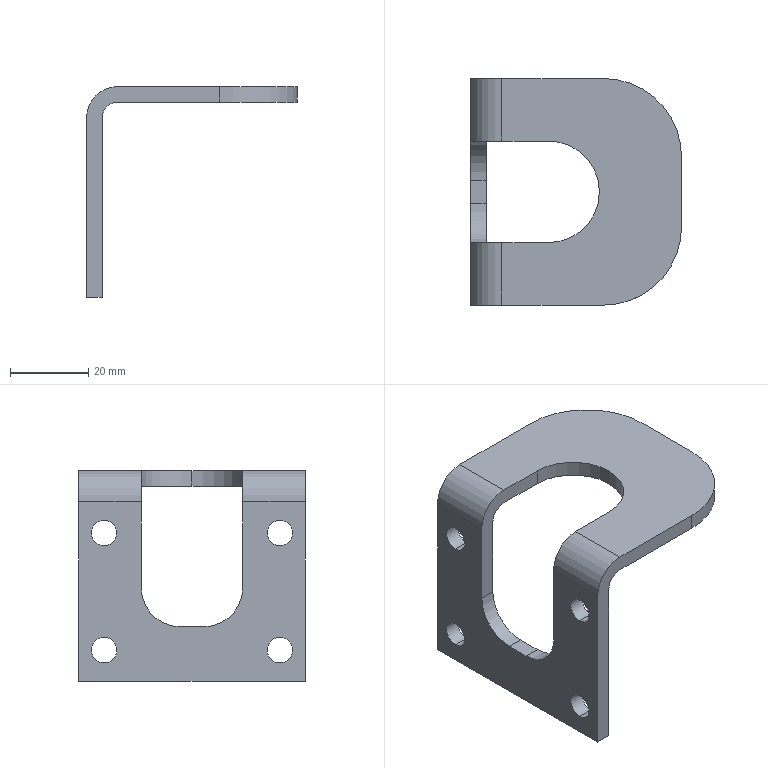Part | STEP file | X77-02002 | 1 solid | 29 faces | box 54 x 58 x 54 mm | volume 15867 mm3 | cylinder 18 | plane 11 | commonest cylinder face diameters 6.5 x8 8 x2 16 x2 20 x2 26 x2 40 x2
STEP:
#1=CARTESIAN_POINT('',(-63.245,51.5,31.345));
#2=VERTEX_POINT('',#1);
#3=CARTESIAN_POINT('',(-63.245,51.5,24.845));
#4=VERTEX_POINT('',#3);
#5=CARTESIAN_POINT('',(-63.245,51.5,28.095));
#6=DIRECTION('',(1.,0.,0.));
#7=DIRECTION('',(0.,0.,-1.));
#8=AXIS2_PLACEMENT_3D('',#5,#6,#7);
#9=CIRCLE('',#8,3.25);
#10=EDGE_CURVE('',#2,#4,#9,.T.);
#11=ORIENTED_EDGE('',*,*,#10,.F.);
#12=CARTESIAN_POINT('',(-59.245,51.5,31.345));
#13=VERTEX_POINT('',#12);
#14=CARTESIAN_POINT('',(-69.245,51.5,31.345));
#15=DIRECTION('',(1.,0.,0.));
#16=VECTOR('',#15,1000.);
#17=LINE('',#14,#16);
#18=EDGE_CURVE('',#2,#13,#17,.T.);
#19=ORIENTED_EDGE('',*,*,#18,.T.);
#20=CARTESIAN_POINT('',(-59.245,51.5,24.845));
#21=VERTEX_POINT('',#20);
#22=CARTESIAN_POINT('',(-59.245,51.5,28.095));
#23=DIRECTION('',(1.,0.,0.));
#24=DIRECTION('',(0.,0.,-1.));
#25=AXIS2_PLACEMENT_3D('',#22,#23,#24);
#26=CIRCLE('',#25,3.25);
#27=EDGE_CURVE('',#13,#21,#26,.T.);
#28=ORIENTED_EDGE('',*,*,#27,.T.);
#29=CARTESIAN_POINT('',(-69.245,51.5,24.845));
#30=DIRECTION('',(1.,0.,0.));
#31=VECTOR('',#30,1000.);
#32=LINE('',#29,#31);
#33=EDGE_CURVE('',#4,#21,#32,.T.);
#34=ORIENTED_EDGE('',*,*,#33,.F.);
#35=EDGE_LOOP('',(#11,#19,#28,#34));
#36=FACE_OUTER_BOUND('',#35,.T.);
#37=CARTESIAN_POINT('',(-69.245,51.5,28.095));
#38=DIRECTION('',(1.,0.,0.));
#39=DIRECTION('',(0.,0.,-1.));
#40=AXIS2_PLACEMENT_3D('',#37,#38,#39);
#41=CYLINDRICAL_SURFACE('',#40,3.25);
#42=ADVANCED_FACE('',(#36),#41,.F.);
#43=CARTESIAN_POINT('',(-63.245,6.5,31.345));
#44=VERTEX_POINT('',#43);
#45=CARTESIAN_POINT('',(-63.245,6.5,24.845));
#46=VERTEX_POINT('',#45);
#47=CARTESIAN_POINT('',(-63.245,6.5,28.095));
#48=DIRECTION('',(1.,0.,0.));
#49=DIRECTION('',(0.,0.,-1.));
#50=AXIS2_PLACEMENT_3D('',#47,#48,#49);
#51=CIRCLE('',#50,3.25);
#52=EDGE_CURVE('',#44,#46,#51,.T.);
#53=ORIENTED_EDGE('',*,*,#52,.F.);
#54=CARTESIAN_POINT('',(-59.245,6.5,31.345));
#55=VERTEX_POINT('',#54);
#56=CARTESIAN_POINT('',(-69.245,6.5,31.345));
#57=DIRECTION('',(1.,0.,0.));
#58=VECTOR('',#57,1000.);
#59=LINE('',#56,#58);
#60=EDGE_CURVE('',#44,#55,#59,.T.);
#61=ORIENTED_EDGE('',*,*,#60,.T.);
#62=CARTESIAN_POINT('',(-59.245,6.5,24.845));
#63=VERTEX_POINT('',#62);
#64=CARTESIAN_POINT('',(-59.245,6.5,28.095));
#65=DIRECTION('',(1.,0.,0.));
#66=DIRECTION('',(0.,0.,-1.));
#67=AXIS2_PLACEMENT_3D('',#64,#65,#66);
#68=CIRCLE('',#67,3.25);
#69=EDGE_CURVE('',#55,#63,#68,.T.);
#70=ORIENTED_EDGE('',*,*,#69,.T.);
#71=CARTESIAN_POINT('',(-69.245,6.5,24.845));
#72=DIRECTION('',(1.,0.,0.));
#73=VECTOR('',#72,1000.);
#74=LINE('',#71,#73);
#75=EDGE_CURVE('',#46,#63,#74,.T.);
#76=ORIENTED_EDGE('',*,*,#75,.F.);
#77=EDGE_LOOP('',(#53,#61,#70,#76));
#78=FACE_OUTER_BOUND('',#77,.T.);
#79=CARTESIAN_POINT('',(-69.245,6.5,28.095));
#80=DIRECTION('',(1.,0.,0.));
#81=DIRECTION('',(0.,0.,-1.));
#82=AXIS2_PLACEMENT_3D('',#79,#80,#81);
#83=CYLINDRICAL_SURFACE('',#82,3.25);
#84=ADVANCED_FACE('',(#78),#83,.F.);
#85=CARTESIAN_POINT('',(-63.245,6.5,1.345));
#86=VERTEX_POINT('',#85);
#87=CARTESIAN_POINT('',(-63.245,6.5,-5.155));
#88=VERTEX_POINT('',#87);
#89=CARTESIAN_POINT('',(-63.245,6.5,-1.905));
#90=DIRECTION('',(1.,0.,0.));
#91=DIRECTION('',(0.,0.,-1.));
#92=AXIS2_PLACEMENT_3D('',#89,#90,#91);
#93=CIRCLE('',#92,3.25);
#94=EDGE_CURVE('',#86,#88,#93,.T.);
#95=ORIENTED_EDGE('',*,*,#94,.F.);
#96=CARTESIAN_POINT('',(-59.245,6.5,1.345));
#97=VERTEX_POINT('',#96);
#98=CARTESIAN_POINT('',(-69.245,6.5,1.345));
#99=DIRECTION('',(1.,0.,0.));
#100=VECTOR('',#99,1000.);
#101=LINE('',#98,#100);
#102=EDGE_CURVE('',#86,#97,#101,.T.);
#103=ORIENTED_EDGE('',*,*,#102,.T.);
#104=CARTESIAN_POINT('',(-59.245,6.5,-5.155));
#105=VERTEX_POINT('',#104);
#106=CARTESIAN_POINT('',(-59.245,6.5,-1.905));
#107=DIRECTION('',(1.,0.,0.));
#108=DIRECTION('',(0.,0.,-1.));
#109=AXIS2_PLACEMENT_3D('',#106,#107,#108);
#110=CIRCLE('',#109,3.25);
#111=EDGE_CURVE('',#97,#105,#110,.T.);
#112=ORIENTED_EDGE('',*,*,#111,.T.);
#113=CARTESIAN_POINT('',(-69.245,6.5,-5.155));
#114=DIRECTION('',(1.,0.,0.));
#115=VECTOR('',#114,1000.);
#116=LINE('',#113,#115);
#117=EDGE_CURVE('',#88,#105,#116,.T.);
#118=ORIENTED_EDGE('',*,*,#117,.F.);
#119=EDGE_LOOP('',(#95,#103,#112,#118));
#120=FACE_OUTER_BOUND('',#119,.T.);
#121=CARTESIAN_POINT('',(-69.245,6.5,-1.905));
#122=DIRECTION('',(1.,0.,0.));
#123=DIRECTION('',(0.,0.,-1.));
#124=AXIS2_PLACEMENT_3D('',#121,#122,#123);
#125=CYLINDRICAL_SURFACE('',#124,3.25);
#126=ADVANCED_FACE('',(#120),#125,.F.);
#127=CARTESIAN_POINT('',(-63.245,51.5,1.345));
#128=VERTEX_POINT('',#127);
#129=CARTESIAN_POINT('',(-63.245,51.5,-5.155));
#130=VERTEX_POINT('',#129);
#131=CARTESIAN_POINT('',(-63.245,51.5,-1.905));
#132=DIRECTION('',(1.,0.,0.));
#133=DIRECTION('',(0.,0.,-1.));
#134=AXIS2_PLACEMENT_3D('',#131,#132,#133);
#135=CIRCLE('',#134,3.25);
#136=EDGE_CURVE('',#128,#130,#135,.T.);
#137=ORIENTED_EDGE('',*,*,#136,.F.);
#138=CARTESIAN_POINT('',(-59.245,51.5,1.345));
#139=VERTEX_POINT('',#138);
#140=CARTESIAN_POINT('',(-69.245,51.5,1.345));
#141=DIRECTION('',(1.,0.,0.));
#142=VECTOR('',#141,1000.);
#143=LINE('',#140,#142);
#144=EDGE_CURVE('',#128,#139,#143,.T.);
#145=ORIENTED_EDGE('',*,*,#144,.T.);
#146=CARTESIAN_POINT('',(-59.245,51.5,-5.155));
#147=VERTEX_POINT('',#146);
#148=CARTESIAN_POINT('',(-59.245,51.5,-1.905));
#149=DIRECTION('',(1.,0.,0.));
#150=DIRECTION('',(0.,0.,-1.));
#151=AXIS2_PLACEMENT_3D('',#148,#149,#150);
#152=CIRCLE('',#151,3.25);
#153=EDGE_CURVE('',#139,#147,#152,.T.);
#154=ORIENTED_EDGE('',*,*,#153,.T.);
#155=CARTESIAN_POINT('',(-69.245,51.5,-5.155));
#156=DIRECTION('',(1.,0.,0.));
#157=VECTOR('',#156,1000.);
#158=LINE('',#155,#157);
#159=EDGE_CURVE('',#130,#147,#158,.T.);
#160=ORIENTED_EDGE('',*,*,#159,.F.);
#161=EDGE_LOOP('',(#137,#145,#154,#160));
#162=FACE_OUTER_BOUND('',#161,.T.);
#163=CARTESIAN_POINT('',(-69.245,51.5,-1.905));
#164=DIRECTION('',(1.,0.,0.));
#165=DIRECTION('',(0.,0.,-1.));
#166=AXIS2_PLACEMENT_3D('',#163,#164,#165);
#167=CYLINDRICAL_SURFACE('',#166,3.25);
#168=ADVANCED_FACE('',(#162),#167,.F.);
#169=CARTESIAN_POINT('',(-30.245,29.,40.095));
#170=VERTEX_POINT('',#169);
#171=CARTESIAN_POINT('',(-43.245,42.,40.095));
#172=VERTEX_POINT('',#171);
#173=CARTESIAN_POINT('',(-43.245,29.,40.095));
#174=DIRECTION('',(0.,0.,1.));
#175=DIRECTION('',(1.,0.,0.));
#176=AXIS2_PLACEMENT_3D('',#173,#174,#175);
#177=CIRCLE('',#176,13.);
#178=EDGE_CURVE('',#170,#172,#177,.T.);
#179=ORIENTED_EDGE('',*,*,#178,.F.);
#180=CARTESIAN_POINT('',(-30.245,29.,44.095));
#181=VERTEX_POINT('',#180);
#182=CARTESIAN_POINT('',(-30.245,29.,4.095));
#183=DIRECTION('',(0.,0.,1.));
#184=VECTOR('',#183,1000.);
#185=LINE('',#182,#184);
#186=EDGE_CURVE('',#170,#181,#185,.T.);
#187=ORIENTED_EDGE('',*,*,#186,.T.);
#188=CARTESIAN_POINT('',(-43.245,42.,44.095));
#189=VERTEX_POINT('',#188);
#190=CARTESIAN_POINT('',(-43.245,29.,44.095));
#191=DIRECTION('',(0.,0.,1.));
#192=DIRECTION('',(1.,0.,0.));
#193=AXIS2_PLACEMENT_3D('',#190,#191,#192);
#194=CIRCLE('',#193,13.);
#195=EDGE_CURVE('',#181,#189,#194,.T.);
#196=ORIENTED_EDGE('',*,*,#195,.T.);
#197=CARTESIAN_POINT('',(-43.245,42.,4.095));
#198=DIRECTION('',(0.,0.,1.));
#199=VECTOR('',#198,1000.);
#200=LINE('',#197,#199);
#201=EDGE_CURVE('',#172,#189,#200,.T.);
#202=ORIENTED_EDGE('',*,*,#201,.F.);
#203=EDGE_LOOP('',(#179,#187,#196,#202));
#204=FACE_OUTER_BOUND('',#203,.T.);
#205=CARTESIAN_POINT('',(-43.245,29.,4.095));
#206=DIRECTION('',(0.,0.,1.));
#207=DIRECTION('',(1.,0.,0.));
#208=AXIS2_PLACEMENT_3D('',#205,#206,#207);
#209=CYLINDRICAL_SURFACE('',#208,13.);
#210=ADVANCED_FACE('',(#204),#209,.F.);
#211=CARTESIAN_POINT('',(-63.245,58.,36.095));
#212=VERTEX_POINT('',#211);
#213=CARTESIAN_POINT('',(-63.245,42.,36.095));
#214=VERTEX_POINT('',#213);
#215=CARTESIAN_POINT('',(-63.245,58.,36.095));
#216=DIRECTION('',(0.,-1.,0.));
#217=VECTOR('',#216,1000.);
#218=LINE('',#215,#217);
#219=EDGE_CURVE('',#212,#214,#218,.T.);
#220=ORIENTED_EDGE('',*,*,#219,.T.);
#221=CARTESIAN_POINT('',(-55.245,42.,44.095));
#222=VERTEX_POINT('',#221);
#223=CARTESIAN_POINT('',(-55.245,42.,36.095));
#224=DIRECTION('',(0.,1.,0.));
#225=DIRECTION('',(0.,0.,1.));
#226=AXIS2_PLACEMENT_3D('',#223,#224,#225);
#227=CIRCLE('',#226,8.);
#228=EDGE_CURVE('',#214,#222,#227,.T.);
#229=ORIENTED_EDGE('',*,*,#228,.T.);
#230=CARTESIAN_POINT('',(-55.245,58.,44.095));
#231=VERTEX_POINT('',#230);
#232=CARTESIAN_POINT('',(-55.245,58.,44.095));
#233=DIRECTION('',(0.,-1.,0.));
#234=VECTOR('',#233,1000.);
#235=LINE('',#232,#234);
#236=EDGE_CURVE('',#231,#222,#235,.T.);
#237=ORIENTED_EDGE('',*,*,#236,.F.);
#238=CARTESIAN_POINT('',(-55.245,58.,36.095));
#239=DIRECTION('',(0.,1.,0.));
#240=DIRECTION('',(0.,0.,-1.));
#241=AXIS2_PLACEMENT_3D('',#238,#239,#240);
#242=CIRCLE('',#241,8.);
#243=EDGE_CURVE('',#212,#231,#242,.T.);
#244=ORIENTED_EDGE('',*,*,#243,.F.);
#245=EDGE_LOOP('',(#220,#229,#237,#244));
#246=FACE_OUTER_BOUND('',#245,.T.);
#247=CARTESIAN_POINT('',(-55.245,58.,36.095));
#248=DIRECTION('',(0.,-1.,0.));
#249=DIRECTION('',(0.,0.,-1.));
#250=AXIS2_PLACEMENT_3D('',#247,#248,#249);
#251=CYLINDRICAL_SURFACE('',#250,8.);
#252=ADVANCED_FACE('',(#246),#251,.T.);
#253=CARTESIAN_POINT('',(-55.245,58.,40.095));
#254=VERTEX_POINT('',#253);
#255=CARTESIAN_POINT('',(-55.245,42.,40.095));
#256=VERTEX_POINT('',#255);
#257=CARTESIAN_POINT('',(-55.245,58.,40.095));
#258=DIRECTION('',(0.,-1.,0.));
#259=VECTOR('',#258,1000.);
#260=LINE('',#257,#259);
#261=EDGE_CURVE('',#254,#256,#260,.T.);
#262=ORIENTED_EDGE('',*,*,#261,.T.);
#263=CARTESIAN_POINT('',(-59.245,42.,36.095));
#264=VERTEX_POINT('',#263);
#265=CARTESIAN_POINT('',(-55.245,42.,36.095));
#266=DIRECTION('',(0.,-1.,0.));
#267=DIRECTION('',(0.,0.,1.));
#268=AXIS2_PLACEMENT_3D('',#265,#266,#267);
#269=CIRCLE('',#268,4.);
#270=EDGE_CURVE('',#256,#264,#269,.T.);
#271=ORIENTED_EDGE('',*,*,#270,.T.);
#272=CARTESIAN_POINT('',(-59.245,58.,36.095));
#273=VERTEX_POINT('',#272);
#274=CARTESIAN_POINT('',(-59.245,58.,36.095));
#275=DIRECTION('',(0.,-1.,0.));
#276=VECTOR('',#275,1000.);
#277=LINE('',#274,#276);
#278=EDGE_CURVE('',#273,#264,#277,.T.);
#279=ORIENTED_EDGE('',*,*,#278,.F.);
#280=CARTESIAN_POINT('',(-55.245,58.,36.095));
#281=DIRECTION('',(0.,-1.,0.));
#282=DIRECTION('',(0.,0.,-1.));
#283=AXIS2_PLACEMENT_3D('',#280,#281,#282);
#284=CIRCLE('',#283,4.);
#285=EDGE_CURVE('',#254,#273,#284,.T.);
#286=ORIENTED_EDGE('',*,*,#285,.F.);
#287=EDGE_LOOP('',(#262,#271,#279,#286));
#288=FACE_OUTER_BOUND('',#287,.T.);
#289=CARTESIAN_POINT('',(-55.245,58.,36.095));
#290=DIRECTION('',(0.,-1.,0.));
#291=DIRECTION('',(0.,0.,-1.));
#292=AXIS2_PLACEMENT_3D('',#289,#290,#291);
#293=CYLINDRICAL_SURFACE('',#292,4.);
#294=ADVANCED_FACE('',(#288),#293,.F.);
#295=CARTESIAN_POINT('',(-59.245,0.,-9.905));
#296=VERTEX_POINT('',#295);
#297=CARTESIAN_POINT('',(-63.245,0.,-9.905));
#298=VERTEX_POINT('',#297);
#299=CARTESIAN_POINT('',(-59.245,0.,-9.905));
#300=DIRECTION('',(-1.,0.,0.));
#301=VECTOR('',#300,1000.);
#302=LINE('',#299,#301);
#303=EDGE_CURVE('',#296,#298,#302,.T.);
#304=ORIENTED_EDGE('',*,*,#303,.T.);
#305=CARTESIAN_POINT('',(-63.245,58.,-9.905));
#306=VERTEX_POINT('',#305);
#307=CARTESIAN_POINT('',(-63.245,58.,-9.905));
#308=DIRECTION('',(0.,-1.,0.));
#309=VECTOR('',#308,1000.);
#310=LINE('',#307,#309);
#311=EDGE_CURVE('',#306,#298,#310,.T.);
#312=ORIENTED_EDGE('',*,*,#311,.F.);
#313=CARTESIAN_POINT('',(-59.245,58.,-9.905));
#314=VERTEX_POINT('',#313);
#315=CARTESIAN_POINT('',(-59.245,58.,-9.905));
#316=DIRECTION('',(-1.,0.,0.));
#317=VECTOR('',#316,1000.);
#318=LINE('',#315,#317);
#319=EDGE_CURVE('',#314,#306,#318,.T.);
#320=ORIENTED_EDGE('',*,*,#319,.F.);
#321=CARTESIAN_POINT('',(-59.245,58.,-9.905));
#322=DIRECTION('',(0.,-1.,0.));
#323=VECTOR('',#322,1000.);
#324=LINE('',#321,#323);
#325=EDGE_CURVE('',#314,#296,#324,.T.);
#326=ORIENTED_EDGE('',*,*,#325,.T.);
#327=EDGE_LOOP('',(#304,#312,#320,#326));
#328=FACE_OUTER_BOUND('',#327,.T.);
#329=CARTESIAN_POINT('',(-59.245,58.,-9.905));
#330=DIRECTION('',(0.,0.,1.));
#331=DIRECTION('',(1.,0.,0.));
#332=AXIS2_PLACEMENT_3D('',#329,#330,#331);
#333=PLANE('',#332);
#334=ADVANCED_FACE('',(#328),#333,.F.);
#335=CARTESIAN_POINT('',(-63.245,51.5,28.095));
#336=DIRECTION('',(1.,0.,0.));
#337=DIRECTION('',(0.,0.,-1.));
#338=AXIS2_PLACEMENT_3D('',#335,#336,#337);
#339=CIRCLE('',#338,3.25);
#340=EDGE_CURVE('',#4,#2,#339,.T.);
#341=ORIENTED_EDGE('',*,*,#340,.T.);
#342=ORIENTED_EDGE('',*,*,#10,.T.);
#343=EDGE_LOOP('',(#341,#342));
#344=FACE_BOUND('',#343,.T.);
#345=CARTESIAN_POINT('',(-63.245,6.5,28.095));
#346=DIRECTION('',(1.,0.,0.));
#347=DIRECTION('',(0.,0.,-1.));
#348=AXIS2_PLACEMENT_3D('',#345,#346,#347);
#349=CIRCLE('',#348,3.25);
#350=EDGE_CURVE('',#46,#44,#349,.T.);
#351=ORIENTED_EDGE('',*,*,#350,.T.);
#352=ORIENTED_EDGE('',*,*,#52,.T.);
#353=EDGE_LOOP('',(#351,#352));
#354=FACE_BOUND('',#353,.T.);
#355=CARTESIAN_POINT('',(-63.245,6.5,-1.905));
#356=DIRECTION('',(1.,0.,0.));
#357=DIRECTION('',(0.,0.,-1.));
#358=AXIS2_PLACEMENT_3D('',#355,#356,#357);
#359=CIRCLE('',#358,3.25);
#360=EDGE_CURVE('',#88,#86,#359,.T.);
#361=ORIENTED_EDGE('',*,*,#360,.T.);
#362=ORIENTED_EDGE('',*,*,#94,.T.);
#363=EDGE_LOOP('',(#361,#362));
#364=FACE_BOUND('',#363,.T.);
#365=CARTESIAN_POINT('',(-63.245,51.5,-1.905));
#366=DIRECTION('',(1.,0.,0.));
#367=DIRECTION('',(0.,0.,-1.));
#368=AXIS2_PLACEMENT_3D('',#365,#366,#367);
#369=CIRCLE('',#368,3.25);
#370=EDGE_CURVE('',#130,#128,#369,.T.);
#371=ORIENTED_EDGE('',*,*,#370,.T.);
#372=ORIENTED_EDGE('',*,*,#136,.T.);
#373=EDGE_LOOP('',(#371,#372));
#374=FACE_BOUND('',#373,.T.);
#375=CARTESIAN_POINT('',(-63.245,32.,4.095));
#376=VERTEX_POINT('',#375);
#377=CARTESIAN_POINT('',(-63.245,26.,4.095));
#378=VERTEX_POINT('',#377);
#379=CARTESIAN_POINT('',(-63.245,58.,4.095));
#380=DIRECTION('',(0.,-1.,0.));
#381=VECTOR('',#380,1000.);
#382=LINE('',#379,#381);
#383=EDGE_CURVE('',#376,#378,#382,.T.);
#384=ORIENTED_EDGE('',*,*,#383,.F.);
#385=CARTESIAN_POINT('',(-63.245,42.,14.095));
#386=VERTEX_POINT('',#385);
#387=CARTESIAN_POINT('',(-63.245,32.,14.095));
#388=DIRECTION('',(1.,0.,0.));
#389=DIRECTION('',(0.,0.,-1.));
#390=AXIS2_PLACEMENT_3D('',#387,#388,#389);
#391=CIRCLE('',#390,10.);
#392=EDGE_CURVE('',#376,#386,#391,.T.);
#393=ORIENTED_EDGE('',*,*,#392,.T.);
#394=CARTESIAN_POINT('',(-63.245,42.,4.095));
#395=DIRECTION('',(0.,0.,1.));
#396=VECTOR('',#395,1000.);
#397=LINE('',#394,#396);
#398=EDGE_CURVE('',#386,#214,#397,.T.);
#399=ORIENTED_EDGE('',*,*,#398,.T.);
#400=ORIENTED_EDGE('',*,*,#219,.F.);
#401=CARTESIAN_POINT('',(-63.245,58.,-9.905));
#402=DIRECTION('',(0.,0.,1.));
#403=VECTOR('',#402,1000.);
#404=LINE('',#401,#403);
#405=EDGE_CURVE('',#306,#212,#404,.T.);
#406=ORIENTED_EDGE('',*,*,#405,.F.);
#407=ORIENTED_EDGE('',*,*,#311,.T.);
#408=CARTESIAN_POINT('',(-63.245,0.,36.095));
#409=VERTEX_POINT('',#408);
#410=CARTESIAN_POINT('',(-63.245,0.,-9.905));
#411=DIRECTION('',(0.,0.,1.));
#412=VECTOR('',#411,1000.);
#413=LINE('',#410,#412);
#414=EDGE_CURVE('',#298,#409,#413,.T.);
#415=ORIENTED_EDGE('',*,*,#414,.T.);
#416=CARTESIAN_POINT('',(-63.245,16.,36.095));
#417=VERTEX_POINT('',#416);
#418=CARTESIAN_POINT('',(-63.245,58.,36.095));
#419=DIRECTION('',(0.,-1.,0.));
#420=VECTOR('',#419,1000.);
#421=LINE('',#418,#420);
#422=EDGE_CURVE('',#417,#409,#421,.T.);
#423=ORIENTED_EDGE('',*,*,#422,.F.);
#424=CARTESIAN_POINT('',(-63.245,16.,14.095));
#425=VERTEX_POINT('',#424);
#426=CARTESIAN_POINT('',(-63.245,16.,4.095));
#427=DIRECTION('',(0.,0.,1.));
#428=VECTOR('',#427,1000.);
#429=LINE('',#426,#428);
#430=EDGE_CURVE('',#425,#417,#429,.T.);
#431=ORIENTED_EDGE('',*,*,#430,.F.);
#432=CARTESIAN_POINT('',(-63.245,26.,14.095));
#433=DIRECTION('',(1.,0.,0.));
#434=DIRECTION('',(0.,0.,-1.));
#435=AXIS2_PLACEMENT_3D('',#432,#433,#434);
#436=CIRCLE('',#435,10.);
#437=EDGE_CURVE('',#425,#378,#436,.T.);
#438=ORIENTED_EDGE('',*,*,#437,.T.);
#439=EDGE_LOOP('',(#384,#393,#399,#400,#406,#407,#415,#423,#431,#438));
#440=FACE_OUTER_BOUND('',#439,.T.);
#441=CARTESIAN_POINT('',(-63.245,58.,-9.905));
#442=DIRECTION('',(1.,0.,0.));
#443=DIRECTION('',(0.,0.,-1.));
#444=AXIS2_PLACEMENT_3D('',#441,#442,#443);
#445=PLANE('',#444);
#446=ADVANCED_FACE('',(#344,#354,#364,#374,#440),#445,.F.);
#447=CARTESIAN_POINT('',(-55.245,16.,44.095));
#448=VERTEX_POINT('',#447);
#449=CARTESIAN_POINT('',(-55.245,0.,44.095));
#450=VERTEX_POINT('',#449);
#451=CARTESIAN_POINT('',(-55.245,58.,44.095));
#452=DIRECTION('',(0.,-1.,0.));
#453=VECTOR('',#452,1000.);
#454=LINE('',#451,#453);
#455=EDGE_CURVE('',#448,#450,#454,.T.);
#456=ORIENTED_EDGE('',*,*,#455,.F.);
#457=CARTESIAN_POINT('',(-55.245,16.,36.095));
#458=DIRECTION('',(0.,-1.,0.));
#459=DIRECTION('',(0.,0.,-1.));
#460=AXIS2_PLACEMENT_3D('',#457,#458,#459);
#461=CIRCLE('',#460,8.);
#462=EDGE_CURVE('',#448,#417,#461,.T.);
#463=ORIENTED_EDGE('',*,*,#462,.T.);
#464=ORIENTED_EDGE('',*,*,#422,.T.);
#465=CARTESIAN_POINT('',(-55.245,0.,36.095));
#466=DIRECTION('',(0.,1.,0.));
#467=DIRECTION('',(0.,0.,-1.));
#468=AXIS2_PLACEMENT_3D('',#465,#466,#467);
#469=CIRCLE('',#468,8.);
#470=EDGE_CURVE('',#409,#450,#469,.T.);
#471=ORIENTED_EDGE('',*,*,#470,.T.);
#472=EDGE_LOOP('',(#456,#463,#464,#471));
#473=FACE_OUTER_BOUND('',#472,.T.);
#474=CARTESIAN_POINT('',(-55.245,58.,36.095));
#475=DIRECTION('',(0.,-1.,0.));
#476=DIRECTION('',(0.,0.,-1.));
#477=AXIS2_PLACEMENT_3D('',#474,#475,#476);
#478=CYLINDRICAL_SURFACE('',#477,8.);
#479=ADVANCED_FACE('',(#473),#478,.T.);
#480=CARTESIAN_POINT('',(-29.245,0.,44.095));
#481=VERTEX_POINT('',#480);
#482=CARTESIAN_POINT('',(-55.245,0.,44.095));
#483=DIRECTION('',(1.,0.,0.));
#484=VECTOR('',#483,1000.);
#485=LINE('',#482,#484);
#486=EDGE_CURVE('',#450,#481,#485,.T.);
#487=ORIENTED_EDGE('',*,*,#486,.T.);
#488=CARTESIAN_POINT('',(-9.245,20.,44.095));
#489=VERTEX_POINT('',#488);
#490=CARTESIAN_POINT('',(-29.245,20.,44.095));
#491=DIRECTION('',(0.,0.,1.));
#492=DIRECTION('',(-1.,0.,0.));
#493=AXIS2_PLACEMENT_3D('',#490,#491,#492);
#494=CIRCLE('',#493,20.);
#495=EDGE_CURVE('',#481,#489,#494,.T.);
#496=ORIENTED_EDGE('',*,*,#495,.T.);
#497=CARTESIAN_POINT('',(-9.245,38.,44.095));
#498=VERTEX_POINT('',#497);
#499=CARTESIAN_POINT('',(-9.245,58.,44.095));
#500=DIRECTION('',(0.,-1.,0.));
#501=VECTOR('',#500,1000.);
#502=LINE('',#499,#501);
#503=EDGE_CURVE('',#498,#489,#502,.T.);
#504=ORIENTED_EDGE('',*,*,#503,.F.);
#505=CARTESIAN_POINT('',(-29.245,58.,44.095));
#506=VERTEX_POINT('',#505);
#507=CARTESIAN_POINT('',(-29.245,38.,44.095));
#508=DIRECTION('',(0.,0.,1.));
#509=DIRECTION('',(-1.,0.,0.));
#510=AXIS2_PLACEMENT_3D('',#507,#508,#509);
#511=CIRCLE('',#510,20.);
#512=EDGE_CURVE('',#498,#506,#511,.T.);
#513=ORIENTED_EDGE('',*,*,#512,.T.);
#514=CARTESIAN_POINT('',(-55.245,58.,44.095));
#515=DIRECTION('',(1.,0.,0.));
#516=VECTOR('',#515,1000.);
#517=LINE('',#514,#516);
#518=EDGE_CURVE('',#231,#506,#517,.T.);
#519=ORIENTED_EDGE('',*,*,#518,.F.);
#520=ORIENTED_EDGE('',*,*,#236,.T.);
#521=CARTESIAN_POINT('',(-63.245,42.,44.095));
#522=DIRECTION('',(-1.,0.,0.));
#523=VECTOR('',#522,1000.);
#524=LINE('',#521,#523);
#525=EDGE_CURVE('',#189,#222,#524,.T.);
#526=ORIENTED_EDGE('',*,*,#525,.F.);
#527=ORIENTED_EDGE('',*,*,#195,.F.);
#528=CARTESIAN_POINT('',(-43.245,16.,44.095));
#529=VERTEX_POINT('',#528);
#530=CARTESIAN_POINT('',(-43.245,29.,44.095));
#531=DIRECTION('',(0.,0.,1.));
#532=DIRECTION('',(1.,0.,0.));
#533=AXIS2_PLACEMENT_3D('',#530,#531,#532);
#534=CIRCLE('',#533,13.);
#535=EDGE_CURVE('',#529,#181,#534,.T.);
#536=ORIENTED_EDGE('',*,*,#535,.F.);
#537=CARTESIAN_POINT('',(-63.245,16.,44.095));
#538=DIRECTION('',(1.,0.,0.));
#539=VECTOR('',#538,1000.);
#540=LINE('',#537,#539);
#541=EDGE_CURVE('',#448,#529,#540,.T.);
#542=ORIENTED_EDGE('',*,*,#541,.F.);
#543=ORIENTED_EDGE('',*,*,#455,.T.);
#544=EDGE_LOOP('',(#487,#496,#504,#513,#519,#520,#526,#527,#536,#542,#543));
#545=FACE_OUTER_BOUND('',#544,.T.);
#546=CARTESIAN_POINT('',(-55.245,58.,44.095));
#547=DIRECTION('',(0.,0.,-1.));
#548=DIRECTION('',(-1.,0.,0.));
#549=AXIS2_PLACEMENT_3D('',#546,#547,#548);
#550=PLANE('',#549);
#551=ADVANCED_FACE('',(#545),#550,.F.);
#552=ORIENTED_EDGE('',*,*,#503,.T.);
#553=CARTESIAN_POINT('',(-9.245,20.,40.095));
#554=VERTEX_POINT('',#553);
#555=CARTESIAN_POINT('',(-9.245,20.,40.095));
#556=DIRECTION('',(0.,0.,-1.));
#557=VECTOR('',#556,1000.);
#558=LINE('',#555,#557);
#559=EDGE_CURVE('',#489,#554,#558,.T.);
#560=ORIENTED_EDGE('',*,*,#559,.T.);
#561=CARTESIAN_POINT('',(-9.245,38.,40.095));
#562=VERTEX_POINT('',#561);
#563=CARTESIAN_POINT('',(-9.245,58.,40.095));
#564=DIRECTION('',(0.,-1.,0.));
#565=VECTOR('',#564,1000.);
#566=LINE('',#563,#565);
#567=EDGE_CURVE('',#562,#554,#566,.T.);
#568=ORIENTED_EDGE('',*,*,#567,.F.);
#569=CARTESIAN_POINT('',(-9.245,38.,44.095));
#570=DIRECTION('',(0.,0.,1.));
#571=VECTOR('',#570,1000.);
#572=LINE('',#569,#571);
#573=EDGE_CURVE('',#562,#498,#572,.T.);
#574=ORIENTED_EDGE('',*,*,#573,.T.);
#575=EDGE_LOOP('',(#552,#560,#568,#574));
#576=FACE_OUTER_BOUND('',#575,.T.);
#577=CARTESIAN_POINT('',(-9.245,58.,44.095));
#578=DIRECTION('',(-1.,0.,0.));
#579=DIRECTION('',(0.,0.,1.));
#580=AXIS2_PLACEMENT_3D('',#577,#578,#579);
#581=PLANE('',#580);
#582=ADVANCED_FACE('',(#576),#581,.F.);
#583=ORIENTED_EDGE('',*,*,#567,.T.);
#584=CARTESIAN_POINT('',(-29.245,0.,40.095));
#585=VERTEX_POINT('',#584);
#586=CARTESIAN_POINT('',(-29.245,20.,40.095));
#587=DIRECTION('',(0.,0.,-1.));
#588=DIRECTION('',(1.,0.,0.));
#589=AXIS2_PLACEMENT_3D('',#586,#587,#588);
#590=CIRCLE('',#589,20.);
#591=EDGE_CURVE('',#554,#585,#590,.T.);
#592=ORIENTED_EDGE('',*,*,#591,.T.);
#593=CARTESIAN_POINT('',(-55.245,0.,40.095));
#594=VERTEX_POINT('',#593);
#595=CARTESIAN_POINT('',(-55.245,0.,40.095));
#596=DIRECTION('',(-1.,0.,0.));
#597=VECTOR('',#596,1000.);
#598=LINE('',#595,#597);
#599=EDGE_CURVE('',#585,#594,#598,.T.);
#600=ORIENTED_EDGE('',*,*,#599,.T.);
#601=CARTESIAN_POINT('',(-55.245,16.,40.095));
#602=VERTEX_POINT('',#601);
#603=CARTESIAN_POINT('',(-55.245,58.,40.095));
#604=DIRECTION('',(0.,-1.,0.));
#605=VECTOR('',#604,1000.);
#606=LINE('',#603,#605);
#607=EDGE_CURVE('',#602,#594,#606,.T.);
#608=ORIENTED_EDGE('',*,*,#607,.F.);
#609=CARTESIAN_POINT('',(-43.245,16.,40.095));
#610=VERTEX_POINT('',#609);
#611=CARTESIAN_POINT('',(-55.245,16.,40.095));
#612=DIRECTION('',(1.,0.,0.));
#613=VECTOR('',#612,1000.);
#614=LINE('',#611,#613);
#615=EDGE_CURVE('',#602,#610,#614,.T.);
#616=ORIENTED_EDGE('',*,*,#615,.T.);
#617=CARTESIAN_POINT('',(-43.245,29.,40.095));
#618=DIRECTION('',(0.,0.,1.));
#619=DIRECTION('',(1.,0.,0.));
#620=AXIS2_PLACEMENT_3D('',#617,#618,#619);
#621=CIRCLE('',#620,13.);
#622=EDGE_CURVE('',#610,#170,#621,.T.);
#623=ORIENTED_EDGE('',*,*,#622,.T.);
#624=ORIENTED_EDGE('',*,*,#178,.T.);
#625=CARTESIAN_POINT('',(-55.245,42.,40.095));
#626=DIRECTION('',(-1.,0.,0.));
#627=VECTOR('',#626,1000.);
#628=LINE('',#625,#627);
#629=EDGE_CURVE('',#172,#256,#628,.T.);
#630=ORIENTED_EDGE('',*,*,#629,.T.);
#631=ORIENTED_EDGE('',*,*,#261,.F.);
#632=CARTESIAN_POINT('',(-29.245,58.,40.095));
#633=VERTEX_POINT('',#632);
#634=CARTESIAN_POINT('',(-55.245,58.,40.095));
#635=DIRECTION('',(-1.,0.,0.));
#636=VECTOR('',#635,1000.);
#637=LINE('',#634,#636);
#638=EDGE_CURVE('',#633,#254,#637,.T.);
#639=ORIENTED_EDGE('',*,*,#638,.F.);
#640=CARTESIAN_POINT('',(-29.245,38.,40.095));
#641=DIRECTION('',(0.,0.,-1.));
#642=DIRECTION('',(1.,0.,0.));
#643=AXIS2_PLACEMENT_3D('',#640,#641,#642);
#644=CIRCLE('',#643,20.);
#645=EDGE_CURVE('',#633,#562,#644,.T.);
#646=ORIENTED_EDGE('',*,*,#645,.T.);
#647=EDGE_LOOP('',(#583,#592,#600,#608,#616,#623,#624,#630,#631,#639,#646));
#648=FACE_OUTER_BOUND('',#647,.T.);
#649=CARTESIAN_POINT('',(-55.245,58.,40.095));
#650=DIRECTION('',(0.,0.,1.));
#651=DIRECTION('',(1.,0.,0.));
#652=AXIS2_PLACEMENT_3D('',#649,#650,#651);
#653=PLANE('',#652);
#654=ADVANCED_FACE('',(#648),#653,.F.);
#655=CARTESIAN_POINT('',(-59.245,16.,36.095));
#656=VERTEX_POINT('',#655);
#657=CARTESIAN_POINT('',(-59.245,0.,36.095));
#658=VERTEX_POINT('',#657);
#659=CARTESIAN_POINT('',(-59.245,58.,36.095));
#660=DIRECTION('',(0.,-1.,0.));
#661=VECTOR('',#660,1000.);
#662=LINE('',#659,#661);
#663=EDGE_CURVE('',#656,#658,#662,.T.);
#664=ORIENTED_EDGE('',*,*,#663,.F.);
#665=CARTESIAN_POINT('',(-55.245,16.,36.095));
#666=DIRECTION('',(0.,1.,0.));
#667=DIRECTION('',(0.,0.,-1.));
#668=AXIS2_PLACEMENT_3D('',#665,#666,#667);
#669=CIRCLE('',#668,4.);
#670=EDGE_CURVE('',#656,#602,#669,.T.);
#671=ORIENTED_EDGE('',*,*,#670,.T.);
#672=ORIENTED_EDGE('',*,*,#607,.T.);
#673=CARTESIAN_POINT('',(-55.245,0.,36.095));
#674=DIRECTION('',(0.,-1.,0.));
#675=DIRECTION('',(0.,0.,-1.));
#676=AXIS2_PLACEMENT_3D('',#673,#674,#675);
#677=CIRCLE('',#676,4.);
#678=EDGE_CURVE('',#594,#658,#677,.T.);
#679=ORIENTED_EDGE('',*,*,#678,.T.);
#680=EDGE_LOOP('',(#664,#671,#672,#679));
#681=FACE_OUTER_BOUND('',#680,.T.);
#682=CARTESIAN_POINT('',(-55.245,58.,36.095));
#683=DIRECTION('',(0.,-1.,0.));
#684=DIRECTION('',(0.,0.,-1.));
#685=AXIS2_PLACEMENT_3D('',#682,#683,#684);
#686=CYLINDRICAL_SURFACE('',#685,4.);
#687=ADVANCED_FACE('',(#681),#686,.F.);
#688=CARTESIAN_POINT('',(-59.245,51.5,28.095));
#689=DIRECTION('',(1.,0.,0.));
#690=DIRECTION('',(0.,0.,-1.));
#691=AXIS2_PLACEMENT_3D('',#688,#689,#690);
#692=CIRCLE('',#691,3.25);
#693=EDGE_CURVE('',#21,#13,#692,.T.);
#694=ORIENTED_EDGE('',*,*,#693,.F.);
#695=ORIENTED_EDGE('',*,*,#27,.F.);
#696=EDGE_LOOP('',(#694,#695));
#697=FACE_BOUND('',#696,.T.);
#698=CARTESIAN_POINT('',(-59.245,6.5,28.095));
#699=DIRECTION('',(1.,0.,0.));
#700=DIRECTION('',(0.,0.,-1.));
#701=AXIS2_PLACEMENT_3D('',#698,#699,#700);
#702=CIRCLE('',#701,3.25);
#703=EDGE_CURVE('',#63,#55,#702,.T.);
#704=ORIENTED_EDGE('',*,*,#703,.F.);
#705=ORIENTED_EDGE('',*,*,#69,.F.);
#706=EDGE_LOOP('',(#704,#705));
#707=FACE_BOUND('',#706,.T.);
#708=CARTESIAN_POINT('',(-59.245,6.5,-1.905));
#709=DIRECTION('',(1.,0.,0.));
#710=DIRECTION('',(0.,0.,-1.));
#711=AXIS2_PLACEMENT_3D('',#708,#709,#710);
#712=CIRCLE('',#711,3.25);
#713=EDGE_CURVE('',#105,#97,#712,.T.);
#714=ORIENTED_EDGE('',*,*,#713,.F.);
#715=ORIENTED_EDGE('',*,*,#111,.F.);
#716=EDGE_LOOP('',(#714,#715));
#717=FACE_BOUND('',#716,.T.);
#718=CARTESIAN_POINT('',(-59.245,51.5,-1.905));
#719=DIRECTION('',(1.,0.,0.));
#720=DIRECTION('',(0.,0.,-1.));
#721=AXIS2_PLACEMENT_3D('',#718,#719,#720);
#722=CIRCLE('',#721,3.25);
#723=EDGE_CURVE('',#147,#139,#722,.T.);
#724=ORIENTED_EDGE('',*,*,#723,.F.);
#725=ORIENTED_EDGE('',*,*,#153,.F.);
#726=EDGE_LOOP('',(#724,#725));
#727=FACE_BOUND('',#726,.T.);
#728=ORIENTED_EDGE('',*,*,#278,.T.);
#729=CARTESIAN_POINT('',(-59.245,42.,14.095));
#730=VERTEX_POINT('',#729);
#731=CARTESIAN_POINT('',(-59.245,42.,-9.905));
#732=DIRECTION('',(0.,0.,-1.));
#733=VECTOR('',#732,1000.);
#734=LINE('',#731,#733);
#735=EDGE_CURVE('',#264,#730,#734,.T.);
#736=ORIENTED_EDGE('',*,*,#735,.T.);
#737=CARTESIAN_POINT('',(-59.245,32.,4.095));
#738=VERTEX_POINT('',#737);
#739=CARTESIAN_POINT('',(-59.245,32.,14.095));
#740=DIRECTION('',(-1.,0.,0.));
#741=DIRECTION('',(0.,0.,1.));
#742=AXIS2_PLACEMENT_3D('',#739,#740,#741);
#743=CIRCLE('',#742,10.);
#744=EDGE_CURVE('',#730,#738,#743,.T.);
#745=ORIENTED_EDGE('',*,*,#744,.T.);
#746=CARTESIAN_POINT('',(-59.245,26.,4.095));
#747=VERTEX_POINT('',#746);
#748=CARTESIAN_POINT('',(-59.245,58.,4.095));
#749=DIRECTION('',(0.,1.,0.));
#750=VECTOR('',#749,1000.);
#751=LINE('',#748,#750);
#752=EDGE_CURVE('',#747,#738,#751,.T.);
#753=ORIENTED_EDGE('',*,*,#752,.F.);
#754=CARTESIAN_POINT('',(-59.245,16.,14.095));
#755=VERTEX_POINT('',#754);
#756=CARTESIAN_POINT('',(-59.245,26.,14.095));
#757=DIRECTION('',(-1.,0.,0.));
#758=DIRECTION('',(0.,0.,1.));
#759=AXIS2_PLACEMENT_3D('',#756,#757,#758);
#760=CIRCLE('',#759,10.);
#761=EDGE_CURVE('',#747,#755,#760,.T.);
#762=ORIENTED_EDGE('',*,*,#761,.T.);
#763=CARTESIAN_POINT('',(-59.245,16.,-9.905));
#764=DIRECTION('',(0.,0.,1.));
#765=VECTOR('',#764,1000.);
#766=LINE('',#763,#765);
#767=EDGE_CURVE('',#755,#656,#766,.T.);
#768=ORIENTED_EDGE('',*,*,#767,.T.);
#769=ORIENTED_EDGE('',*,*,#663,.T.);
#770=CARTESIAN_POINT('',(-59.245,0.,-9.905));
#771=DIRECTION('',(0.,0.,-1.));
#772=VECTOR('',#771,1000.);
#773=LINE('',#770,#772);
#774=EDGE_CURVE('',#658,#296,#773,.T.);
#775=ORIENTED_EDGE('',*,*,#774,.T.);
#776=ORIENTED_EDGE('',*,*,#325,.F.);
#777=CARTESIAN_POINT('',(-59.245,58.,-9.905));
#778=DIRECTION('',(0.,0.,-1.));
#779=VECTOR('',#778,1000.);
#780=LINE('',#777,#779);
#781=EDGE_CURVE('',#273,#314,#780,.T.);
#782=ORIENTED_EDGE('',*,*,#781,.F.);
#783=EDGE_LOOP('',(#728,#736,#745,#753,#762,#768,#769,#775,#776,#782));
#784=FACE_OUTER_BOUND('',#783,.T.);
#785=CARTESIAN_POINT('',(-59.245,58.,-9.905));
#786=DIRECTION('',(-1.,0.,0.));
#787=DIRECTION('',(0.,0.,1.));
#788=AXIS2_PLACEMENT_3D('',#785,#786,#787);
#789=PLANE('',#788);
#790=ADVANCED_FACE('',(#697,#707,#717,#727,#784),#789,.F.);
#791=ORIENTED_EDGE('',*,*,#518,.T.);
#792=CARTESIAN_POINT('',(-29.245,58.,36.095));
#793=DIRECTION('',(0.,0.,-1.));
#794=VECTOR('',#793,1000.);
#795=LINE('',#792,#794);
#796=EDGE_CURVE('',#506,#633,#795,.T.);
#797=ORIENTED_EDGE('',*,*,#796,.T.);
#798=ORIENTED_EDGE('',*,*,#638,.T.);
#799=ORIENTED_EDGE('',*,*,#285,.T.);
#800=ORIENTED_EDGE('',*,*,#781,.T.);
#801=ORIENTED_EDGE('',*,*,#319,.T.);
#802=ORIENTED_EDGE('',*,*,#405,.T.);
#803=ORIENTED_EDGE('',*,*,#243,.T.);
#804=EDGE_LOOP('',(#791,#797,#798,#799,#800,#801,#802,#803));
#805=FACE_OUTER_BOUND('',#804,.T.);
#806=CARTESIAN_POINT('',(-55.245,58.,36.095));
#807=DIRECTION('',(0.,-1.,0.));
#808=DIRECTION('',(0.,0.,-1.));
#809=AXIS2_PLACEMENT_3D('',#806,#807,#808);
#810=PLANE('',#809);
#811=ADVANCED_FACE('',(#805),#810,.F.);
#812=ORIENTED_EDGE('',*,*,#599,.F.);
#813=CARTESIAN_POINT('',(-29.245,0.,44.095));
#814=DIRECTION('',(0.,0.,1.));
#815=VECTOR('',#814,1000.);
#816=LINE('',#813,#815);
#817=EDGE_CURVE('',#585,#481,#816,.T.);
#818=ORIENTED_EDGE('',*,*,#817,.T.);
#819=ORIENTED_EDGE('',*,*,#486,.F.);
#820=ORIENTED_EDGE('',*,*,#470,.F.);
#821=ORIENTED_EDGE('',*,*,#414,.F.);
#822=ORIENTED_EDGE('',*,*,#303,.F.);
#823=ORIENTED_EDGE('',*,*,#774,.F.);
#824=ORIENTED_EDGE('',*,*,#678,.F.);
#825=EDGE_LOOP('',(#812,#818,#819,#820,#821,#822,#823,#824));
#826=FACE_OUTER_BOUND('',#825,.T.);
#827=CARTESIAN_POINT('',(-55.245,0.,36.095));
#828=DIRECTION('',(0.,-1.,0.));
#829=DIRECTION('',(0.,0.,-1.));
#830=AXIS2_PLACEMENT_3D('',#827,#828,#829);
#831=PLANE('',#830);
#832=ADVANCED_FACE('',(#826),#831,.T.);
#833=ORIENTED_EDGE('',*,*,#186,.F.);
#834=ORIENTED_EDGE('',*,*,#622,.F.);
#835=CARTESIAN_POINT('',(-43.245,16.,4.095));
#836=DIRECTION('',(0.,0.,1.));
#837=VECTOR('',#836,1000.);
#838=LINE('',#835,#837);
#839=EDGE_CURVE('',#610,#529,#838,.T.);
#840=ORIENTED_EDGE('',*,*,#839,.T.);
#841=ORIENTED_EDGE('',*,*,#535,.T.);
#842=EDGE_LOOP('',(#833,#834,#840,#841));
#843=FACE_OUTER_BOUND('',#842,.T.);
#844=CARTESIAN_POINT('',(-43.245,29.,4.095));
#845=DIRECTION('',(0.,0.,1.));
#846=DIRECTION('',(1.,0.,0.));
#847=AXIS2_PLACEMENT_3D('',#844,#845,#846);
#848=CYLINDRICAL_SURFACE('',#847,13.);
#849=ADVANCED_FACE('',(#843),#848,.F.);
#850=ORIENTED_EDGE('',*,*,#398,.F.);
#851=CARTESIAN_POINT('',(-63.245,42.,14.095));
#852=DIRECTION('',(1.,0.,0.));
#853=VECTOR('',#852,1000.);
#854=LINE('',#851,#853);
#855=EDGE_CURVE('',#386,#730,#854,.T.);
#856=ORIENTED_EDGE('',*,*,#855,.T.);
#857=ORIENTED_EDGE('',*,*,#735,.F.);
#858=ORIENTED_EDGE('',*,*,#270,.F.);
#859=ORIENTED_EDGE('',*,*,#629,.F.);
#860=ORIENTED_EDGE('',*,*,#201,.T.);
#861=ORIENTED_EDGE('',*,*,#525,.T.);
#862=ORIENTED_EDGE('',*,*,#228,.F.);
#863=EDGE_LOOP('',(#850,#856,#857,#858,#859,#860,#861,#862));
#864=FACE_OUTER_BOUND('',#863,.T.);
#865=CARTESIAN_POINT('',(-63.245,42.,4.095));
#866=DIRECTION('',(0.,1.,0.));
#867=DIRECTION('',(0.,0.,1.));
#868=AXIS2_PLACEMENT_3D('',#865,#866,#867);
#869=PLANE('',#868);
#870=ADVANCED_FACE('',(#864),#869,.F.);
#871=ORIENTED_EDGE('',*,*,#767,.F.);
#872=CARTESIAN_POINT('',(-63.245,16.,14.095));
#873=DIRECTION('',(-1.,0.,0.));
#874=VECTOR('',#873,1000.);
#875=LINE('',#872,#874);
#876=EDGE_CURVE('',#755,#425,#875,.T.);
#877=ORIENTED_EDGE('',*,*,#876,.T.);
#878=ORIENTED_EDGE('',*,*,#430,.T.);
#879=ORIENTED_EDGE('',*,*,#462,.F.);
#880=ORIENTED_EDGE('',*,*,#541,.T.);
#881=ORIENTED_EDGE('',*,*,#839,.F.);
#882=ORIENTED_EDGE('',*,*,#615,.F.);
#883=ORIENTED_EDGE('',*,*,#670,.F.);
#884=EDGE_LOOP('',(#871,#877,#878,#879,#880,#881,#882,#883));
#885=FACE_OUTER_BOUND('',#884,.T.);
#886=CARTESIAN_POINT('',(-63.245,16.,4.095));
#887=DIRECTION('',(0.,-1.,0.));
#888=DIRECTION('',(0.,0.,-1.));
#889=AXIS2_PLACEMENT_3D('',#886,#887,#888);
#890=PLANE('',#889);
#891=ADVANCED_FACE('',(#885),#890,.F.);
#892=ORIENTED_EDGE('',*,*,#383,.T.);
#893=CARTESIAN_POINT('',(-63.245,26.,4.095));
#894=DIRECTION('',(1.,0.,0.));
#895=VECTOR('',#894,1000.);
#896=LINE('',#893,#895);
#897=EDGE_CURVE('',#378,#747,#896,.T.);
#898=ORIENTED_EDGE('',*,*,#897,.T.);
#899=ORIENTED_EDGE('',*,*,#752,.T.);
#900=CARTESIAN_POINT('',(-63.245,32.,4.095));
#901=DIRECTION('',(-1.,0.,0.));
#902=VECTOR('',#901,1000.);
#903=LINE('',#900,#902);
#904=EDGE_CURVE('',#738,#376,#903,.T.);
#905=ORIENTED_EDGE('',*,*,#904,.T.);
#906=EDGE_LOOP('',(#892,#898,#899,#905));
#907=FACE_OUTER_BOUND('',#906,.T.);
#908=CARTESIAN_POINT('',(-63.245,29.,4.095));
#909=DIRECTION('',(0.,0.,1.));
#910=DIRECTION('',(1.,0.,0.));
#911=AXIS2_PLACEMENT_3D('',#908,#909,#910);
#912=PLANE('',#911);
#913=ADVANCED_FACE('',(#907),#912,.T.);
#914=ORIENTED_EDGE('',*,*,#495,.F.);
#915=ORIENTED_EDGE('',*,*,#817,.F.);
#916=ORIENTED_EDGE('',*,*,#591,.F.);
#917=ORIENTED_EDGE('',*,*,#559,.F.);
#918=EDGE_LOOP('',(#914,#915,#916,#917));
#919=FACE_OUTER_BOUND('',#918,.T.);
#920=CARTESIAN_POINT('',(-29.245,20.,44.095));
#921=DIRECTION('',(0.,0.,1.));
#922=DIRECTION('',(1.,0.,0.));
#923=AXIS2_PLACEMENT_3D('',#920,#921,#922);
#924=CYLINDRICAL_SURFACE('',#923,20.);
#925=ADVANCED_FACE('',(#919),#924,.T.);
#926=ORIENTED_EDGE('',*,*,#512,.F.);
#927=ORIENTED_EDGE('',*,*,#573,.F.);
#928=ORIENTED_EDGE('',*,*,#645,.F.);
#929=ORIENTED_EDGE('',*,*,#796,.F.);
#930=EDGE_LOOP('',(#926,#927,#928,#929));
#931=FACE_OUTER_BOUND('',#930,.T.);
#932=CARTESIAN_POINT('',(-29.245,38.,36.095));
#933=DIRECTION('',(0.,0.,-1.));
#934=DIRECTION('',(-1.,0.,0.));
#935=AXIS2_PLACEMENT_3D('',#932,#933,#934);
#936=CYLINDRICAL_SURFACE('',#935,20.);
#937=ADVANCED_FACE('',(#931),#936,.T.);
#938=ORIENTED_EDGE('',*,*,#144,.F.);
#939=ORIENTED_EDGE('',*,*,#370,.F.);
#940=ORIENTED_EDGE('',*,*,#159,.T.);
#941=ORIENTED_EDGE('',*,*,#723,.T.);
#942=EDGE_LOOP('',(#938,#939,#940,#941));
#943=FACE_OUTER_BOUND('',#942,.T.);
#944=CARTESIAN_POINT('',(-69.245,51.5,-1.905));
#945=DIRECTION('',(1.,0.,0.));
#946=DIRECTION('',(0.,0.,-1.));
#947=AXIS2_PLACEMENT_3D('',#944,#945,#946);
#948=CYLINDRICAL_SURFACE('',#947,3.25);
#949=ADVANCED_FACE('',(#943),#948,.F.);
#950=ORIENTED_EDGE('',*,*,#102,.F.);
#951=ORIENTED_EDGE('',*,*,#360,.F.);
#952=ORIENTED_EDGE('',*,*,#117,.T.);
#953=ORIENTED_EDGE('',*,*,#713,.T.);
#954=EDGE_LOOP('',(#950,#951,#952,#953));
#955=FACE_OUTER_BOUND('',#954,.T.);
#956=CARTESIAN_POINT('',(-69.245,6.5,-1.905));
#957=DIRECTION('',(1.,0.,0.));
#958=DIRECTION('',(0.,0.,-1.));
#959=AXIS2_PLACEMENT_3D('',#956,#957,#958);
#960=CYLINDRICAL_SURFACE('',#959,3.25);
#961=ADVANCED_FACE('',(#955),#960,.F.);
#962=ORIENTED_EDGE('',*,*,#60,.F.);
#963=ORIENTED_EDGE('',*,*,#350,.F.);
#964=ORIENTED_EDGE('',*,*,#75,.T.);
#965=ORIENTED_EDGE('',*,*,#703,.T.);
#966=EDGE_LOOP('',(#962,#963,#964,#965));
#967=FACE_OUTER_BOUND('',#966,.T.);
#968=CARTESIAN_POINT('',(-69.245,6.5,28.095));
#969=DIRECTION('',(1.,0.,0.));
#970=DIRECTION('',(0.,0.,-1.));
#971=AXIS2_PLACEMENT_3D('',#968,#969,#970);
#972=CYLINDRICAL_SURFACE('',#971,3.25);
#973=ADVANCED_FACE('',(#967),#972,.F.);
#974=ORIENTED_EDGE('',*,*,#18,.F.);
#975=ORIENTED_EDGE('',*,*,#340,.F.);
#976=ORIENTED_EDGE('',*,*,#33,.T.);
#977=ORIENTED_EDGE('',*,*,#693,.T.);
#978=EDGE_LOOP('',(#974,#975,#976,#977));
#979=FACE_OUTER_BOUND('',#978,.T.);
#980=CARTESIAN_POINT('',(-69.245,51.5,28.095));
#981=DIRECTION('',(1.,0.,0.));
#982=DIRECTION('',(0.,0.,-1.));
#983=AXIS2_PLACEMENT_3D('',#980,#981,#982);
#984=CYLINDRICAL_SURFACE('',#983,3.25);
#985=ADVANCED_FACE('',(#979),#984,.F.);
#986=ORIENTED_EDGE('',*,*,#437,.F.);
#987=ORIENTED_EDGE('',*,*,#876,.F.);
#988=ORIENTED_EDGE('',*,*,#761,.F.);
#989=ORIENTED_EDGE('',*,*,#897,.F.);
#990=EDGE_LOOP('',(#986,#987,#988,#989));
#991=FACE_OUTER_BOUND('',#990,.T.);
#992=CARTESIAN_POINT('',(-63.245,26.,14.095));
#993=DIRECTION('',(1.,0.,0.));
#994=DIRECTION('',(0.,0.,-1.));
#995=AXIS2_PLACEMENT_3D('',#992,#993,#994);
#996=CYLINDRICAL_SURFACE('',#995,10.);
#997=ADVANCED_FACE('',(#991),#996,.F.);
#998=ORIENTED_EDGE('',*,*,#744,.F.);
#999=ORIENTED_EDGE('',*,*,#855,.F.);
#1000=ORIENTED_EDGE('',*,*,#392,.F.);
#1001=ORIENTED_EDGE('',*,*,#904,.F.);
#1002=EDGE_LOOP('',(#998,#999,#1000,#1001));
#1003=FACE_OUTER_BOUND('',#1002,.T.);
#1004=CARTESIAN_POINT('',(-63.245,32.,14.095));
#1005=DIRECTION('',(-1.,0.,0.));
#1006=DIRECTION('',(0.,0.,1.));
#1007=AXIS2_PLACEMENT_3D('',#1004,#1005,#1006);
#1008=CYLINDRICAL_SURFACE('',#1007,10.);
#1009=ADVANCED_FACE('',(#1003),#1008,.F.);
#1010=CLOSED_SHELL('',(#42,#84,#126,#168,#210,#252,#294,#334,#446,#479,#551,#582,#654,#687,#790,#811,#832,#849,#870,#891,#913,#925,#937,#949,#961,#973,#985,#997,#1009));
#1011=MANIFOLD_SOLID_BREP('',#1010);
#1012=CARTESIAN_POINT('',(0.,0.,0.));
#1013=DIRECTION('',(0.,0.,1.));
#1014=DIRECTION('',(1.,0.,0.));
#1015=AXIS2_PLACEMENT_3D('',#1012,#1013,#1014);
#1016=(LENGTH_UNIT()NAMED_UNIT(*)SI_UNIT(.MILLI.,.METRE.));
#1017=UNCERTAINTY_MEASURE_WITH_UNIT(LENGTH_MEASURE(0.00001),#1016,'','');
#1018=(NAMED_UNIT(*)PLANE_ANGLE_UNIT()SI_UNIT($,.RADIAN.));
#1019=(NAMED_UNIT(*)SI_UNIT($,.STERADIAN.)SOLID_ANGLE_UNIT());
#1020=(GEOMETRIC_REPRESENTATION_CONTEXT(3)GLOBAL_UNCERTAINTY_ASSIGNED_CONTEXT((#1017))GLOBAL_UNIT_ASSIGNED_CONTEXT((#1016,#1018,#1019))REPRESENTATION_CONTEXT('',''));
#1021=ADVANCED_BREP_SHAPE_REPRESENTATION('',(#1011,#1015),#1020);